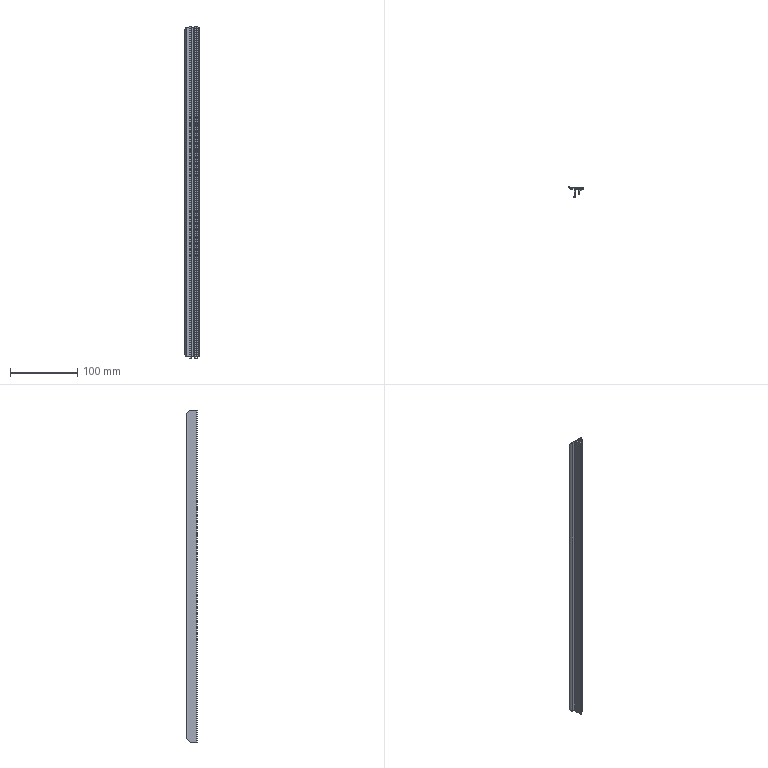Part | NX | features BREP 1 | 1 solid | 43 faces | box 21.266 x 16.173 x 494.9 mm | volume 33584 mm3 | plane 28 | cylinder 15 | commonest cylinder face diameters 0.585 x7 0.4 x2 1.951 x2 1.561 x1 8.16 x1 10.664 x1
STEP:
#1=CARTESIAN_POINT('',(0.,2.699,242.251));
#2=VERTEX_POINT('',#1);
#3=CARTESIAN_POINT('',(2.095,-0.55,245.5));
#4=VERTEX_POINT('',#3);
#5=CARTESIAN_POINT('',(0.,2.699,242.251));
#6=CARTESIAN_POINT('',(0.2706,1.376,243.574));
#7=CARTESIAN_POINT('',(1.002,0.242,244.708));
#8=CARTESIAN_POINT('',(2.095,-0.55,245.5));
#9=(BOUNDED_CURVE()B_SPLINE_CURVE(3,(#5,#6,#7,#8),.UNSPECIFIED.,.F.,.F.)B_SPLINE_CURVE_WITH_KNOTS((4,4),(1.773,2.515),.UNSPECIFIED.)CURVE()GEOMETRIC_REPRESENTATION_ITEM()RATIONAL_B_SPLINE_CURVE((1.,0.9547,0.9547,1.))REPRESENTATION_ITEM(''));
#10=EDGE_CURVE('',#2,#4,#9,.T.);
#11=ORIENTED_EDGE('',*,*,#10,.F.);
#12=CARTESIAN_POINT('',(0.,2.699,-242.251));
#13=VERTEX_POINT('',#12);
#14=CARTESIAN_POINT('',(0.,2.699,247.45));
#15=DIRECTION('',(0.,0.,-1.));
#16=VECTOR('',#15,1000.);
#17=LINE('',#14,#16);
#18=EDGE_CURVE('',#2,#13,#17,.T.);
#19=ORIENTED_EDGE('',*,*,#18,.T.);
#20=CARTESIAN_POINT('',(2.095,-0.55,-245.5));
#21=VERTEX_POINT('',#20);
#22=CARTESIAN_POINT('',(2.095,-0.55,-245.5));
#23=CARTESIAN_POINT('',(1.002,0.242,-244.708));
#24=CARTESIAN_POINT('',(0.2706,1.376,-243.574));
#25=CARTESIAN_POINT('',(0.,2.699,-242.251));
#26=(BOUNDED_CURVE()B_SPLINE_CURVE(3,(#22,#23,#24,#25),.UNSPECIFIED.,.F.,.F.)B_SPLINE_CURVE_WITH_KNOTS((4,4),(0.6271,1.369),.UNSPECIFIED.)CURVE()GEOMETRIC_REPRESENTATION_ITEM()RATIONAL_B_SPLINE_CURVE((1.,0.9547,0.9547,1.))REPRESENTATION_ITEM(''));
#27=EDGE_CURVE('',#21,#13,#26,.T.);
#28=ORIENTED_EDGE('',*,*,#27,.F.);
#29=CARTESIAN_POINT('',(2.095,-0.55,247.45));
#30=DIRECTION('',(0.,0.,-1.));
#31=VECTOR('',#30,1000.);
#32=LINE('',#29,#31);
#33=EDGE_CURVE('',#4,#21,#32,.T.);
#34=ORIENTED_EDGE('',*,*,#33,.F.);
#35=EDGE_LOOP('',(#11,#19,#28,#34));
#36=FACE_BOUND('',#35,.T.);
#37=CARTESIAN_POINT('',(5.224,3.768,247.45));
#38=DIRECTION('',(0.,0.,-1.));
#39=DIRECTION('',(-1.,0.,0.));
#40=AXIS2_PLACEMENT_3D('',#37,#38,#39);
#41=CYLINDRICAL_SURFACE('',#40,5.332);
#42=ADVANCED_FACE('',(#36),#41,.T.);
#43=CARTESIAN_POINT('',(7.9,-0.55,245.5));
#44=VERTEX_POINT('',#43);
#45=CARTESIAN_POINT('',(2.095,-0.55,245.5));
#46=DIRECTION('',(1.,0.,0.));
#47=VECTOR('',#46,1000.);
#48=LINE('',#45,#47);
#49=EDGE_CURVE('',#4,#44,#48,.T.);
#50=ORIENTED_EDGE('',*,*,#49,.F.);
#51=ORIENTED_EDGE('',*,*,#33,.T.);
#52=CARTESIAN_POINT('',(7.9,-0.55,-245.5));
#53=VERTEX_POINT('',#52);
#54=CARTESIAN_POINT('',(2.095,-0.55,-245.5));
#55=DIRECTION('',(-1.,0.,0.));
#56=VECTOR('',#55,1000.);
#57=LINE('',#54,#56);
#58=EDGE_CURVE('',#53,#21,#57,.T.);
#59=ORIENTED_EDGE('',*,*,#58,.F.);
#60=CARTESIAN_POINT('',(7.9,-0.55,247.45));
#61=DIRECTION('',(0.,0.,-1.));
#62=VECTOR('',#61,1000.);
#63=LINE('',#60,#62);
#64=EDGE_CURVE('',#44,#53,#63,.T.);
#65=ORIENTED_EDGE('',*,*,#64,.F.);
#66=EDGE_LOOP('',(#50,#51,#59,#65));
#67=FACE_BOUND('',#66,.T.);
#68=CARTESIAN_POINT('',(2.095,-0.55,247.45));
#69=DIRECTION('',(0.,1.,0.));
#70=DIRECTION('',(1.,0.,0.));
#71=AXIS2_PLACEMENT_3D('',#68,#69,#70);
#72=PLANE('',#71);
#73=ADVANCED_FACE('',(#67),#72,.F.);
#74=CARTESIAN_POINT('',(7.9,-2.5,247.45));
#75=VERTEX_POINT('',#74);
#76=CARTESIAN_POINT('',(7.9,-1.525,246.475));
#77=DIRECTION('',(0.,-0.7071,0.7071));
#78=VECTOR('',#77,1000.);
#79=LINE('',#76,#78);
#80=EDGE_CURVE('',#44,#75,#79,.T.);
#81=ORIENTED_EDGE('',*,*,#80,.F.);
#82=ORIENTED_EDGE('',*,*,#64,.T.);
#83=CARTESIAN_POINT('',(7.9,-2.5,-247.45));
#84=VERTEX_POINT('',#83);
#85=CARTESIAN_POINT('',(7.9,245.925,0.975));
#86=DIRECTION('',(0.,0.7071,0.7071));
#87=VECTOR('',#86,1000.);
#88=LINE('',#85,#87);
#89=EDGE_CURVE('',#84,#53,#88,.T.);
#90=ORIENTED_EDGE('',*,*,#89,.F.);
#91=CARTESIAN_POINT('',(7.9,-11.847,-247.45));
#92=VERTEX_POINT('',#91);
#93=CARTESIAN_POINT('',(7.9,-0.55,-247.45));
#94=DIRECTION('',(0.,-1.,0.));
#95=VECTOR('',#94,1000.);
#96=LINE('',#93,#95);
#97=EDGE_CURVE('',#84,#92,#96,.T.);
#98=ORIENTED_EDGE('',*,*,#97,.T.);
#99=CARTESIAN_POINT('',(7.9,-11.847,247.45));
#100=VERTEX_POINT('',#99);
#101=CARTESIAN_POINT('',(7.9,-11.847,247.45));
#102=DIRECTION('',(0.,0.,-1.));
#103=VECTOR('',#102,1000.);
#104=LINE('',#101,#103);
#105=EDGE_CURVE('',#100,#92,#104,.T.);
#106=ORIENTED_EDGE('',*,*,#105,.F.);
#107=CARTESIAN_POINT('',(7.9,-0.55,247.45));
#108=DIRECTION('',(0.,-1.,0.));
#109=VECTOR('',#108,1000.);
#110=LINE('',#107,#109);
#111=EDGE_CURVE('',#75,#100,#110,.T.);
#112=ORIENTED_EDGE('',*,*,#111,.F.);
#113=EDGE_LOOP('',(#81,#82,#90,#98,#106,#112));
#114=FACE_BOUND('',#113,.T.);
#115=CARTESIAN_POINT('',(7.9,-0.55,247.45));
#116=DIRECTION('',(1.,0.,0.));
#117=DIRECTION('',(0.,1.,0.));
#118=AXIS2_PLACEMENT_3D('',#115,#116,#117);
#119=PLANE('',#118);
#120=ADVANCED_FACE('',(#114),#119,.F.);
#121=CARTESIAN_POINT('',(9.363,-2.5,247.45));
#122=VERTEX_POINT('',#121);
#123=CARTESIAN_POINT('',(9.363,-1.526,246.476));
#124=VERTEX_POINT('',#123);
#125=CARTESIAN_POINT('',(9.363,-7.399,252.349));
#126=DIRECTION('',(0.,0.7071,-0.7071));
#127=VECTOR('',#126,1000.);
#128=LINE('',#125,#127);
#129=EDGE_CURVE('',#122,#124,#128,.T.);
#130=ORIENTED_EDGE('',*,*,#129,.F.);
#131=CARTESIAN_POINT('',(9.363,-12.298,247.45));
#132=VERTEX_POINT('',#131);
#133=CARTESIAN_POINT('',(9.363,-12.298,247.45));
#134=DIRECTION('',(0.,1.,0.));
#135=VECTOR('',#134,1000.);
#136=LINE('',#133,#135);
#137=EDGE_CURVE('',#132,#122,#136,.T.);
#138=ORIENTED_EDGE('',*,*,#137,.F.);
#139=CARTESIAN_POINT('',(9.363,-12.298,-247.45));
#140=VERTEX_POINT('',#139);
#141=CARTESIAN_POINT('',(9.363,-12.298,247.45));
#142=DIRECTION('',(0.,0.,-1.));
#143=VECTOR('',#142,1000.);
#144=LINE('',#141,#143);
#145=EDGE_CURVE('',#132,#140,#144,.T.);
#146=ORIENTED_EDGE('',*,*,#145,.T.);
#147=CARTESIAN_POINT('',(9.363,-2.5,-247.45));
#148=VERTEX_POINT('',#147);
#149=CARTESIAN_POINT('',(9.363,-12.298,-247.45));
#150=DIRECTION('',(0.,1.,0.));
#151=VECTOR('',#150,1000.);
#152=LINE('',#149,#151);
#153=EDGE_CURVE('',#140,#148,#152,.T.);
#154=ORIENTED_EDGE('',*,*,#153,.T.);
#155=CARTESIAN_POINT('',(9.363,-1.526,-246.476));
#156=VERTEX_POINT('',#155);
#157=CARTESIAN_POINT('',(9.363,240.051,-4.899));
#158=DIRECTION('',(0.,-0.7071,-0.7071));
#159=VECTOR('',#158,1000.);
#160=LINE('',#157,#159);
#161=EDGE_CURVE('',#156,#148,#160,.T.);
#162=ORIENTED_EDGE('',*,*,#161,.F.);
#163=CARTESIAN_POINT('',(9.363,-1.526,247.45));
#164=DIRECTION('',(0.,0.,-1.));
#165=VECTOR('',#164,1000.);
#166=LINE('',#163,#165);
#167=EDGE_CURVE('',#124,#156,#166,.T.);
#168=ORIENTED_EDGE('',*,*,#167,.F.);
#169=EDGE_LOOP('',(#130,#138,#146,#154,#162,#168));
#170=FACE_BOUND('',#169,.T.);
#171=CARTESIAN_POINT('',(9.363,-12.298,247.45));
#172=DIRECTION('',(-1.,0.,0.));
#173=DIRECTION('',(0.,0.,1.));
#174=AXIS2_PLACEMENT_3D('',#171,#172,#173);
#175=PLANE('',#174);
#176=ADVANCED_FACE('',(#170),#175,.F.);
#177=CARTESIAN_POINT('',(10.339,-0.55,245.5));
#178=VERTEX_POINT('',#177);
#179=CARTESIAN_POINT('',(9.363,-1.526,246.476));
#180=CARTESIAN_POINT('',(9.363,-0.9541,245.904));
#181=CARTESIAN_POINT('',(9.768,-0.55,245.5));
#182=CARTESIAN_POINT('',(10.339,-0.55,245.5));
#183=(BOUNDED_CURVE()B_SPLINE_CURVE(3,(#179,#180,#181,#182),.UNSPECIFIED.,.F.,.F.)B_SPLINE_CURVE_WITH_KNOTS((4,4),(4.712,6.283),.UNSPECIFIED.)CURVE()GEOMETRIC_REPRESENTATION_ITEM()RATIONAL_B_SPLINE_CURVE((1.,0.8047,0.8047,1.))REPRESENTATION_ITEM(''));
#184=EDGE_CURVE('',#124,#178,#183,.T.);
#185=ORIENTED_EDGE('',*,*,#184,.F.);
#186=ORIENTED_EDGE('',*,*,#167,.T.);
#187=CARTESIAN_POINT('',(10.339,-0.55,-245.5));
#188=VERTEX_POINT('',#187);
#189=CARTESIAN_POINT('',(10.339,-0.55,-245.5));
#190=CARTESIAN_POINT('',(9.768,-0.55,-245.5));
#191=CARTESIAN_POINT('',(9.363,-0.9541,-245.904));
#192=CARTESIAN_POINT('',(9.363,-1.526,-246.476));
#193=(BOUNDED_CURVE()B_SPLINE_CURVE(3,(#189,#190,#191,#192),.UNSPECIFIED.,.F.,.F.)B_SPLINE_CURVE_WITH_KNOTS((4,4),(3.142,4.712),.UNSPECIFIED.)CURVE()GEOMETRIC_REPRESENTATION_ITEM()RATIONAL_B_SPLINE_CURVE((1.,0.8047,0.8047,1.))REPRESENTATION_ITEM(''));
#194=EDGE_CURVE('',#188,#156,#193,.T.);
#195=ORIENTED_EDGE('',*,*,#194,.F.);
#196=CARTESIAN_POINT('',(10.339,-0.55,247.45));
#197=DIRECTION('',(0.,0.,-1.));
#198=VECTOR('',#197,1000.);
#199=LINE('',#196,#198);
#200=EDGE_CURVE('',#178,#188,#199,.T.);
#201=ORIENTED_EDGE('',*,*,#200,.F.);
#202=EDGE_LOOP('',(#185,#186,#195,#201));
#203=FACE_BOUND('',#202,.T.);
#204=CARTESIAN_POINT('',(10.339,-1.526,247.45));
#205=DIRECTION('',(0.,0.,-1.));
#206=DIRECTION('',(-1.,0.,0.));
#207=AXIS2_PLACEMENT_3D('',#204,#205,#206);
#208=CYLINDRICAL_SURFACE('',#207,0.9756);
#209=ADVANCED_FACE('',(#203),#208,.F.);
#210=CARTESIAN_POINT('',(13.461,-0.55,245.5));
#211=VERTEX_POINT('',#210);
#212=CARTESIAN_POINT('',(10.339,-0.55,245.5));
#213=DIRECTION('',(1.,0.,0.));
#214=VECTOR('',#213,1000.);
#215=LINE('',#212,#214);
#216=EDGE_CURVE('',#178,#211,#215,.T.);
#217=ORIENTED_EDGE('',*,*,#216,.F.);
#218=ORIENTED_EDGE('',*,*,#200,.T.);
#219=CARTESIAN_POINT('',(13.461,-0.55,-245.5));
#220=VERTEX_POINT('',#219);
#221=CARTESIAN_POINT('',(10.339,-0.55,-245.5));
#222=DIRECTION('',(-1.,0.,0.));
#223=VECTOR('',#222,1000.);
#224=LINE('',#221,#223);
#225=EDGE_CURVE('',#220,#188,#224,.T.);
#226=ORIENTED_EDGE('',*,*,#225,.F.);
#227=CARTESIAN_POINT('',(13.461,-0.55,247.45));
#228=DIRECTION('',(0.,0.,-1.));
#229=VECTOR('',#228,1000.);
#230=LINE('',#227,#229);
#231=EDGE_CURVE('',#211,#220,#230,.T.);
#232=ORIENTED_EDGE('',*,*,#231,.F.);
#233=EDGE_LOOP('',(#217,#218,#226,#232));
#234=FACE_BOUND('',#233,.T.);
#235=CARTESIAN_POINT('',(10.339,-0.55,247.45));
#236=DIRECTION('',(0.,1.,0.));
#237=DIRECTION('',(1.,0.,0.));
#238=AXIS2_PLACEMENT_3D('',#235,#236,#237);
#239=PLANE('',#238);
#240=ADVANCED_FACE('',(#234),#239,.F.);
#241=CARTESIAN_POINT('',(14.437,-1.526,246.476));
#242=VERTEX_POINT('',#241);
#243=CARTESIAN_POINT('',(13.461,-0.55,245.5));
#244=CARTESIAN_POINT('',(14.032,-0.55,245.5));
#245=CARTESIAN_POINT('',(14.437,-0.9541,245.904));
#246=CARTESIAN_POINT('',(14.437,-1.526,246.476));
#247=(BOUNDED_CURVE()B_SPLINE_CURVE(3,(#243,#244,#245,#246),.UNSPECIFIED.,.F.,.F.)B_SPLINE_CURVE_WITH_KNOTS((4,4),(0.,1.571),.UNSPECIFIED.)CURVE()GEOMETRIC_REPRESENTATION_ITEM()RATIONAL_B_SPLINE_CURVE((1.,0.8047,0.8047,1.))REPRESENTATION_ITEM(''));
#248=EDGE_CURVE('',#211,#242,#247,.T.);
#249=ORIENTED_EDGE('',*,*,#248,.F.);
#250=ORIENTED_EDGE('',*,*,#231,.T.);
#251=CARTESIAN_POINT('',(14.437,-1.526,-246.476));
#252=VERTEX_POINT('',#251);
#253=CARTESIAN_POINT('',(14.437,-1.526,-246.476));
#254=CARTESIAN_POINT('',(14.437,-0.9541,-245.904));
#255=CARTESIAN_POINT('',(14.032,-0.55,-245.5));
#256=CARTESIAN_POINT('',(13.461,-0.55,-245.5));
#257=(BOUNDED_CURVE()B_SPLINE_CURVE(3,(#253,#254,#255,#256),.UNSPECIFIED.,.F.,.F.)B_SPLINE_CURVE_WITH_KNOTS((4,4),(1.571,3.142),.UNSPECIFIED.)CURVE()GEOMETRIC_REPRESENTATION_ITEM()RATIONAL_B_SPLINE_CURVE((1.,0.8047,0.8047,1.))REPRESENTATION_ITEM(''));
#258=EDGE_CURVE('',#252,#220,#257,.T.);
#259=ORIENTED_EDGE('',*,*,#258,.F.);
#260=CARTESIAN_POINT('',(14.437,-1.526,247.45));
#261=DIRECTION('',(0.,0.,-1.));
#262=VECTOR('',#261,1000.);
#263=LINE('',#260,#262);
#264=EDGE_CURVE('',#242,#252,#263,.T.);
#265=ORIENTED_EDGE('',*,*,#264,.F.);
#266=EDGE_LOOP('',(#249,#250,#259,#265));
#267=FACE_BOUND('',#266,.T.);
#268=CARTESIAN_POINT('',(13.461,-1.526,247.45));
#269=DIRECTION('',(0.,0.,-1.));
#270=DIRECTION('',(-1.,0.,0.));
#271=AXIS2_PLACEMENT_3D('',#268,#269,#270);
#272=CYLINDRICAL_SURFACE('',#271,0.9756);
#273=ADVANCED_FACE('',(#267),#272,.F.);
#274=CARTESIAN_POINT('',(14.437,-2.5,247.45));
#275=VERTEX_POINT('',#274);
#276=CARTESIAN_POINT('',(14.437,-2.013,246.963));
#277=DIRECTION('',(0.,-0.7071,0.7071));
#278=VECTOR('',#277,1000.);
#279=LINE('',#276,#278);
#280=EDGE_CURVE('',#242,#275,#279,.T.);
#281=ORIENTED_EDGE('',*,*,#280,.F.);
#282=ORIENTED_EDGE('',*,*,#264,.T.);
#283=CARTESIAN_POINT('',(14.437,-2.5,-247.45));
#284=VERTEX_POINT('',#283);
#285=CARTESIAN_POINT('',(14.437,245.437,0.4872));
#286=DIRECTION('',(0.,0.7071,0.7071));
#287=VECTOR('',#286,1000.);
#288=LINE('',#285,#287);
#289=EDGE_CURVE('',#284,#252,#288,.T.);
#290=ORIENTED_EDGE('',*,*,#289,.F.);
#291=CARTESIAN_POINT('',(14.437,-8.128,-247.45));
#292=VERTEX_POINT('',#291);
#293=CARTESIAN_POINT('',(14.437,-1.526,-247.45));
#294=DIRECTION('',(0.,-1.,0.));
#295=VECTOR('',#294,1000.);
#296=LINE('',#293,#295);
#297=EDGE_CURVE('',#284,#292,#296,.T.);
#298=ORIENTED_EDGE('',*,*,#297,.T.);
#299=CARTESIAN_POINT('',(14.437,-8.128,247.45));
#300=VERTEX_POINT('',#299);
#301=CARTESIAN_POINT('',(14.437,-8.128,247.45));
#302=DIRECTION('',(0.,0.,-1.));
#303=VECTOR('',#302,1000.);
#304=LINE('',#301,#303);
#305=EDGE_CURVE('',#300,#292,#304,.T.);
#306=ORIENTED_EDGE('',*,*,#305,.F.);
#307=CARTESIAN_POINT('',(14.437,-1.526,247.45));
#308=DIRECTION('',(0.,-1.,0.));
#309=VECTOR('',#308,1000.);
#310=LINE('',#307,#309);
#311=EDGE_CURVE('',#275,#300,#310,.T.);
#312=ORIENTED_EDGE('',*,*,#311,.F.);
#313=EDGE_LOOP('',(#281,#282,#290,#298,#306,#312));
#314=FACE_BOUND('',#313,.T.);
#315=CARTESIAN_POINT('',(14.437,-1.526,247.45));
#316=DIRECTION('',(1.,0.,0.));
#317=DIRECTION('',(0.,1.,0.));
#318=AXIS2_PLACEMENT_3D('',#315,#316,#317);
#319=PLANE('',#318);
#320=ADVANCED_FACE('',(#314),#319,.F.);
#321=CARTESIAN_POINT('',(15.9,-2.5,247.45));
#322=VERTEX_POINT('',#321);
#323=CARTESIAN_POINT('',(15.9,-0.55,245.5));
#324=VERTEX_POINT('',#323);
#325=CARTESIAN_POINT('',(15.9,-4.93,249.88));
#326=DIRECTION('',(0.,0.7071,-0.7071));
#327=VECTOR('',#326,1000.);
#328=LINE('',#325,#327);
#329=EDGE_CURVE('',#322,#324,#328,.T.);
#330=ORIENTED_EDGE('',*,*,#329,.F.);
#331=CARTESIAN_POINT('',(15.9,-7.36,247.45));
#332=VERTEX_POINT('',#331);
#333=CARTESIAN_POINT('',(15.9,-7.36,247.45));
#334=DIRECTION('',(0.,1.,0.));
#335=VECTOR('',#334,1000.);
#336=LINE('',#333,#335);
#337=EDGE_CURVE('',#332,#322,#336,.T.);
#338=ORIENTED_EDGE('',*,*,#337,.F.);
#339=CARTESIAN_POINT('',(15.9,-7.36,-247.45));
#340=VERTEX_POINT('',#339);
#341=CARTESIAN_POINT('',(15.9,-7.36,247.45));
#342=DIRECTION('',(0.,0.,-1.));
#343=VECTOR('',#342,1000.);
#344=LINE('',#341,#343);
#345=EDGE_CURVE('',#332,#340,#344,.T.);
#346=ORIENTED_EDGE('',*,*,#345,.T.);
#347=CARTESIAN_POINT('',(15.9,-2.5,-247.45));
#348=VERTEX_POINT('',#347);
#349=CARTESIAN_POINT('',(15.9,-7.36,-247.45));
#350=DIRECTION('',(0.,1.,0.));
#351=VECTOR('',#350,1000.);
#352=LINE('',#349,#351);
#353=EDGE_CURVE('',#340,#348,#352,.T.);
#354=ORIENTED_EDGE('',*,*,#353,.T.);
#355=CARTESIAN_POINT('',(15.9,-0.55,-245.5));
#356=VERTEX_POINT('',#355);
#357=CARTESIAN_POINT('',(15.9,242.52,-2.43));
#358=DIRECTION('',(0.,-0.7071,-0.7071));
#359=VECTOR('',#358,1000.);
#360=LINE('',#357,#359);
#361=EDGE_CURVE('',#356,#348,#360,.T.);
#362=ORIENTED_EDGE('',*,*,#361,.F.);
#363=CARTESIAN_POINT('',(15.9,-0.55,247.45));
#364=DIRECTION('',(0.,0.,-1.));
#365=VECTOR('',#364,1000.);
#366=LINE('',#363,#365);
#367=EDGE_CURVE('',#324,#356,#366,.T.);
#368=ORIENTED_EDGE('',*,*,#367,.F.);
#369=EDGE_LOOP('',(#330,#338,#346,#354,#362,#368));
#370=FACE_BOUND('',#369,.T.);
#371=CARTESIAN_POINT('',(15.9,-7.36,247.45));
#372=DIRECTION('',(-1.,0.,0.));
#373=DIRECTION('',(0.,0.,1.));
#374=AXIS2_PLACEMENT_3D('',#371,#372,#373);
#375=PLANE('',#374);
#376=ADVANCED_FACE('',(#370),#375,.F.);
#377=CARTESIAN_POINT('',(17.363,-0.55,245.5));
#378=VERTEX_POINT('',#377);
#379=CARTESIAN_POINT('',(15.9,-0.55,245.5));
#380=DIRECTION('',(1.,0.,0.));
#381=VECTOR('',#380,1000.);
#382=LINE('',#379,#381);
#383=EDGE_CURVE('',#324,#378,#382,.T.);
#384=ORIENTED_EDGE('',*,*,#383,.F.);
#385=ORIENTED_EDGE('',*,*,#367,.T.);
#386=CARTESIAN_POINT('',(17.363,-0.55,-245.5));
#387=VERTEX_POINT('',#386);
#388=CARTESIAN_POINT('',(15.9,-0.55,-245.5));
#389=DIRECTION('',(-1.,0.,0.));
#390=VECTOR('',#389,1000.);
#391=LINE('',#388,#390);
#392=EDGE_CURVE('',#387,#356,#391,.T.);
#393=ORIENTED_EDGE('',*,*,#392,.F.);
#394=CARTESIAN_POINT('',(17.363,-0.55,247.45));
#395=DIRECTION('',(0.,0.,-1.));
#396=VECTOR('',#395,1000.);
#397=LINE('',#394,#396);
#398=EDGE_CURVE('',#378,#387,#397,.T.);
#399=ORIENTED_EDGE('',*,*,#398,.F.);
#400=EDGE_LOOP('',(#384,#385,#393,#399));
#401=FACE_BOUND('',#400,.T.);
#402=CARTESIAN_POINT('',(15.9,-0.55,247.45));
#403=DIRECTION('',(0.,1.,0.));
#404=DIRECTION('',(1.,0.,0.));
#405=AXIS2_PLACEMENT_3D('',#402,#403,#404);
#406=PLANE('',#405);
#407=ADVANCED_FACE('',(#401),#406,.F.);
#408=CARTESIAN_POINT('',(17.363,-2.5,247.45));
#409=VERTEX_POINT('',#408);
#410=CARTESIAN_POINT('',(17.363,-1.525,246.475));
#411=DIRECTION('',(0.,-0.7071,0.7071));
#412=VECTOR('',#411,1000.);
#413=LINE('',#410,#412);
#414=EDGE_CURVE('',#378,#409,#413,.T.);
#415=ORIENTED_EDGE('',*,*,#414,.F.);
#416=ORIENTED_EDGE('',*,*,#398,.T.);
#417=CARTESIAN_POINT('',(17.363,-2.5,-247.45));
#418=VERTEX_POINT('',#417);
#419=CARTESIAN_POINT('',(17.363,245.925,0.975));
#420=DIRECTION('',(0.,0.7071,0.7071));
#421=VECTOR('',#420,1000.);
#422=LINE('',#419,#421);
#423=EDGE_CURVE('',#418,#387,#422,.T.);
#424=ORIENTED_EDGE('',*,*,#423,.F.);
#425=CARTESIAN_POINT('',(17.363,-2.501,-247.45));
#426=VERTEX_POINT('',#425);
#427=CARTESIAN_POINT('',(17.363,-0.55,-247.45));
#428=DIRECTION('',(0.,-1.,0.));
#429=VECTOR('',#428,1000.);
#430=LINE('',#427,#429);
#431=EDGE_CURVE('',#418,#426,#430,.T.);
#432=ORIENTED_EDGE('',*,*,#431,.T.);
#433=CARTESIAN_POINT('',(17.363,-2.501,247.45));
#434=VERTEX_POINT('',#433);
#435=CARTESIAN_POINT('',(17.363,-2.501,247.45));
#436=DIRECTION('',(0.,0.,-1.));
#437=VECTOR('',#436,1000.);
#438=LINE('',#435,#437);
#439=EDGE_CURVE('',#434,#426,#438,.T.);
#440=ORIENTED_EDGE('',*,*,#439,.F.);
#441=CARTESIAN_POINT('',(17.363,-0.55,247.45));
#442=DIRECTION('',(0.,-1.,0.));
#443=VECTOR('',#442,1000.);
#444=LINE('',#441,#443);
#445=EDGE_CURVE('',#409,#434,#444,.T.);
#446=ORIENTED_EDGE('',*,*,#445,.F.);
#447=EDGE_LOOP('',(#415,#416,#424,#432,#440,#446));
#448=FACE_BOUND('',#447,.T.);
#449=CARTESIAN_POINT('',(17.363,-0.55,247.45));
#450=DIRECTION('',(1.,0.,0.));
#451=DIRECTION('',(0.,1.,0.));
#452=AXIS2_PLACEMENT_3D('',#449,#450,#451);
#453=PLANE('',#452);
#454=ADVANCED_FACE('',(#448),#453,.F.);
#455=CARTESIAN_POINT('',(19.049,-2.5,247.45));
#456=VERTEX_POINT('',#455);
#457=CARTESIAN_POINT('',(19.315,-2.209,247.159));
#458=VERTEX_POINT('',#457);
#459=CARTESIAN_POINT('',(19.049,-2.5,247.45));
#460=CARTESIAN_POINT('',(19.207,-2.485,247.435));
#461=CARTESIAN_POINT('',(19.315,-2.368,247.318));
#462=CARTESIAN_POINT('',(19.315,-2.209,247.159));
#463=(BOUNDED_CURVE()B_SPLINE_CURVE(3,(#459,#460,#461,#462),.UNSPECIFIED.,.F.,.F.)B_SPLINE_CURVE_WITH_KNOTS((4,4),(3.233,4.712),.UNSPECIFIED.)CURVE()GEOMETRIC_REPRESENTATION_ITEM()RATIONAL_B_SPLINE_CURVE((1.,0.8258,0.8258,1.))REPRESENTATION_ITEM(''));
#464=EDGE_CURVE('',#456,#458,#463,.T.);
#465=ORIENTED_EDGE('',*,*,#464,.F.);
#466=CARTESIAN_POINT('',(19.022,-2.501,247.45));
#467=VERTEX_POINT('',#466);
#468=CARTESIAN_POINT('',(19.022,-2.209,247.45));
#469=DIRECTION('',(0.,0.,1.));
#470=DIRECTION('',(1.,0.,0.));
#471=AXIS2_PLACEMENT_3D('',#468,#469,#470);
#472=CIRCLE('',#471,0.2927);
#473=EDGE_CURVE('',#467,#456,#472,.T.);
#474=ORIENTED_EDGE('',*,*,#473,.F.);
#475=CARTESIAN_POINT('',(19.022,-2.501,-247.45));
#476=VERTEX_POINT('',#475);
#477=CARTESIAN_POINT('',(19.022,-2.501,247.45));
#478=DIRECTION('',(0.,0.,-1.));
#479=VECTOR('',#478,1000.);
#480=LINE('',#477,#479);
#481=EDGE_CURVE('',#467,#476,#480,.T.);
#482=ORIENTED_EDGE('',*,*,#481,.T.);
#483=CARTESIAN_POINT('',(19.049,-2.5,-247.45));
#484=VERTEX_POINT('',#483);
#485=CARTESIAN_POINT('',(19.022,-2.209,-247.45));
#486=DIRECTION('',(0.,0.,1.));
#487=DIRECTION('',(1.,0.,0.));
#488=AXIS2_PLACEMENT_3D('',#485,#486,#487);
#489=CIRCLE('',#488,0.2927);
#490=EDGE_CURVE('',#476,#484,#489,.T.);
#491=ORIENTED_EDGE('',*,*,#490,.T.);
#492=CARTESIAN_POINT('',(19.315,-2.209,-247.159));
#493=VERTEX_POINT('',#492);
#494=CARTESIAN_POINT('',(19.315,-2.209,-247.159));
#495=CARTESIAN_POINT('',(19.315,-2.368,-247.318));
#496=CARTESIAN_POINT('',(19.207,-2.485,-247.435));
#497=CARTESIAN_POINT('',(19.049,-2.5,-247.45));
#498=(BOUNDED_CURVE()B_SPLINE_CURVE(3,(#494,#495,#496,#497),.UNSPECIFIED.,.F.,.F.)B_SPLINE_CURVE_WITH_KNOTS((4,4),(4.712,6.192),.UNSPECIFIED.)CURVE()GEOMETRIC_REPRESENTATION_ITEM()RATIONAL_B_SPLINE_CURVE((1.,0.8258,0.8258,1.))REPRESENTATION_ITEM(''));
#499=EDGE_CURVE('',#493,#484,#498,.T.);
#500=ORIENTED_EDGE('',*,*,#499,.F.);
#501=CARTESIAN_POINT('',(19.315,-2.209,247.45));
#502=DIRECTION('',(0.,0.,-1.));
#503=VECTOR('',#502,1000.);
#504=LINE('',#501,#503);
#505=EDGE_CURVE('',#458,#493,#504,.T.);
#506=ORIENTED_EDGE('',*,*,#505,.F.);
#507=EDGE_LOOP('',(#465,#474,#482,#491,#500,#506));
#508=FACE_BOUND('',#507,.T.);
#509=CARTESIAN_POINT('',(19.022,-2.209,247.45));
#510=DIRECTION('',(0.,0.,-1.));
#511=DIRECTION('',(-1.,0.,0.));
#512=AXIS2_PLACEMENT_3D('',#509,#510,#511);
#513=CYLINDRICAL_SURFACE('',#512,0.2927);
#514=ADVANCED_FACE('',(#508),#513,.T.);
#515=CARTESIAN_POINT('',(19.315,-0.8427,245.793));
#516=VERTEX_POINT('',#515);
#517=CARTESIAN_POINT('',(19.315,-2.354,247.304));
#518=DIRECTION('',(0.,0.7071,-0.7071));
#519=VECTOR('',#518,1000.);
#520=LINE('',#517,#519);
#521=EDGE_CURVE('',#458,#516,#520,.T.);
#522=ORIENTED_EDGE('',*,*,#521,.F.);
#523=ORIENTED_EDGE('',*,*,#505,.T.);
#524=CARTESIAN_POINT('',(19.315,-0.8427,-245.793));
#525=VERTEX_POINT('',#524);
#526=CARTESIAN_POINT('',(19.315,245.096,0.1457));
#527=DIRECTION('',(0.,-0.7071,-0.7071));
#528=VECTOR('',#527,1000.);
#529=LINE('',#526,#528);
#530=EDGE_CURVE('',#525,#493,#529,.T.);
#531=ORIENTED_EDGE('',*,*,#530,.F.);
#532=CARTESIAN_POINT('',(19.315,-0.8427,247.45));
#533=DIRECTION('',(0.,0.,-1.));
#534=VECTOR('',#533,1000.);
#535=LINE('',#532,#534);
#536=EDGE_CURVE('',#516,#525,#535,.T.);
#537=ORIENTED_EDGE('',*,*,#536,.F.);
#538=EDGE_LOOP('',(#522,#523,#531,#537));
#539=FACE_BOUND('',#538,.T.);
#540=CARTESIAN_POINT('',(19.315,-2.209,247.45));
#541=DIRECTION('',(-1.,0.,0.));
#542=DIRECTION('',(0.,0.,1.));
#543=AXIS2_PLACEMENT_3D('',#540,#541,#542);
#544=PLANE('',#543);
#545=ADVANCED_FACE('',(#539),#544,.F.);
#546=CARTESIAN_POINT('',(19.607,-0.55,245.5));
#547=VERTEX_POINT('',#546);
#548=CARTESIAN_POINT('',(19.315,-0.8427,245.793));
#549=CARTESIAN_POINT('',(19.315,-0.6712,245.621));
#550=CARTESIAN_POINT('',(19.436,-0.55,245.5));
#551=CARTESIAN_POINT('',(19.607,-0.55,245.5));
#552=(BOUNDED_CURVE()B_SPLINE_CURVE(3,(#548,#549,#550,#551),.UNSPECIFIED.,.F.,.F.)B_SPLINE_CURVE_WITH_KNOTS((4,4),(4.712,6.283),.UNSPECIFIED.)CURVE()GEOMETRIC_REPRESENTATION_ITEM()RATIONAL_B_SPLINE_CURVE((1.,0.8047,0.8047,1.))REPRESENTATION_ITEM(''));
#553=EDGE_CURVE('',#516,#547,#552,.T.);
#554=ORIENTED_EDGE('',*,*,#553,.F.);
#555=ORIENTED_EDGE('',*,*,#536,.T.);
#556=CARTESIAN_POINT('',(19.607,-0.55,-245.5));
#557=VERTEX_POINT('',#556);
#558=CARTESIAN_POINT('',(19.607,-0.55,-245.5));
#559=CARTESIAN_POINT('',(19.436,-0.55,-245.5));
#560=CARTESIAN_POINT('',(19.315,-0.6712,-245.621));
#561=CARTESIAN_POINT('',(19.315,-0.8427,-245.793));
#562=(BOUNDED_CURVE()B_SPLINE_CURVE(3,(#558,#559,#560,#561),.UNSPECIFIED.,.F.,.F.)B_SPLINE_CURVE_WITH_KNOTS((4,4),(3.142,4.712),.UNSPECIFIED.)CURVE()GEOMETRIC_REPRESENTATION_ITEM()RATIONAL_B_SPLINE_CURVE((1.,0.8047,0.8047,1.))REPRESENTATION_ITEM(''));
#563=EDGE_CURVE('',#557,#525,#562,.T.);
#564=ORIENTED_EDGE('',*,*,#563,.F.);
#565=CARTESIAN_POINT('',(19.607,-0.55,247.45));
#566=DIRECTION('',(0.,0.,-1.));
#567=VECTOR('',#566,1000.);
#568=LINE('',#565,#567);
#569=EDGE_CURVE('',#547,#557,#568,.T.);
#570=ORIENTED_EDGE('',*,*,#569,.F.);
#571=EDGE_LOOP('',(#554,#555,#564,#570));
#572=FACE_BOUND('',#571,.T.);
#573=CARTESIAN_POINT('',(19.607,-0.8427,247.45));
#574=DIRECTION('',(0.,0.,-1.));
#575=DIRECTION('',(-1.,0.,0.));
#576=AXIS2_PLACEMENT_3D('',#573,#574,#575);
#577=CYLINDRICAL_SURFACE('',#576,0.2927);
#578=ADVANCED_FACE('',(#572),#577,.F.);
#579=CARTESIAN_POINT('',(20.973,-0.55,245.5));
#580=VERTEX_POINT('',#579);
#581=CARTESIAN_POINT('',(19.607,-0.55,245.5));
#582=DIRECTION('',(1.,0.,0.));
#583=VECTOR('',#582,1000.);
#584=LINE('',#581,#583);
#585=EDGE_CURVE('',#547,#580,#584,.T.);
#586=ORIENTED_EDGE('',*,*,#585,.F.);
#587=ORIENTED_EDGE('',*,*,#569,.T.);
#588=CARTESIAN_POINT('',(20.973,-0.55,-245.5));
#589=VERTEX_POINT('',#588);
#590=CARTESIAN_POINT('',(19.607,-0.55,-245.5));
#591=DIRECTION('',(-1.,0.,0.));
#592=VECTOR('',#591,1000.);
#593=LINE('',#590,#592);
#594=EDGE_CURVE('',#589,#557,#593,.T.);
#595=ORIENTED_EDGE('',*,*,#594,.F.);
#596=CARTESIAN_POINT('',(20.973,-0.55,247.45));
#597=DIRECTION('',(0.,0.,-1.));
#598=VECTOR('',#597,1000.);
#599=LINE('',#596,#598);
#600=EDGE_CURVE('',#580,#589,#599,.T.);
#601=ORIENTED_EDGE('',*,*,#600,.F.);
#602=EDGE_LOOP('',(#586,#587,#595,#601));
#603=FACE_BOUND('',#602,.T.);
#604=CARTESIAN_POINT('',(19.607,-0.55,247.45));
#605=DIRECTION('',(0.,1.,0.));
#606=DIRECTION('',(1.,0.,0.));
#607=AXIS2_PLACEMENT_3D('',#604,#605,#606);
#608=PLANE('',#607);
#609=ADVANCED_FACE('',(#603),#608,.F.);
#610=CARTESIAN_POINT('',(21.266,-0.2573,245.207));
#611=VERTEX_POINT('',#610);
#612=CARTESIAN_POINT('',(20.973,-0.55,245.5));
#613=CARTESIAN_POINT('',(21.145,-0.55,245.5));
#614=CARTESIAN_POINT('',(21.266,-0.4288,245.379));
#615=CARTESIAN_POINT('',(21.266,-0.2573,245.207));
#616=(BOUNDED_CURVE()B_SPLINE_CURVE(3,(#612,#613,#614,#615),.UNSPECIFIED.,.F.,.F.)B_SPLINE_CURVE_WITH_KNOTS((4,4),(3.142,4.712),.UNSPECIFIED.)CURVE()GEOMETRIC_REPRESENTATION_ITEM()RATIONAL_B_SPLINE_CURVE((1.,0.8047,0.8047,1.))REPRESENTATION_ITEM(''));
#617=EDGE_CURVE('',#580,#611,#616,.T.);
#618=ORIENTED_EDGE('',*,*,#617,.F.);
#619=ORIENTED_EDGE('',*,*,#600,.T.);
#620=CARTESIAN_POINT('',(21.266,-0.2573,-245.207));
#621=VERTEX_POINT('',#620);
#622=CARTESIAN_POINT('',(21.266,-0.2573,-245.207));
#623=CARTESIAN_POINT('',(21.266,-0.4288,-245.379));
#624=CARTESIAN_POINT('',(21.145,-0.55,-245.5));
#625=CARTESIAN_POINT('',(20.973,-0.55,-245.5));
#626=(BOUNDED_CURVE()B_SPLINE_CURVE(3,(#622,#623,#624,#625),.UNSPECIFIED.,.F.,.F.)B_SPLINE_CURVE_WITH_KNOTS((4,4),(4.712,6.283),.UNSPECIFIED.)CURVE()GEOMETRIC_REPRESENTATION_ITEM()RATIONAL_B_SPLINE_CURVE((1.,0.8047,0.8047,1.))REPRESENTATION_ITEM(''));
#627=EDGE_CURVE('',#621,#589,#626,.T.);
#628=ORIENTED_EDGE('',*,*,#627,.F.);
#629=CARTESIAN_POINT('',(21.266,-0.2573,247.45));
#630=DIRECTION('',(0.,0.,-1.));
#631=VECTOR('',#630,1000.);
#632=LINE('',#629,#631);
#633=EDGE_CURVE('',#611,#621,#632,.T.);
#634=ORIENTED_EDGE('',*,*,#633,.F.);
#635=EDGE_LOOP('',(#618,#619,#628,#634));
#636=FACE_BOUND('',#635,.T.);
#637=CARTESIAN_POINT('',(20.973,-0.2573,247.45));
#638=DIRECTION('',(0.,0.,-1.));
#639=DIRECTION('',(-1.,0.,0.));
#640=AXIS2_PLACEMENT_3D('',#637,#638,#639);
#641=CYLINDRICAL_SURFACE('',#640,0.2927);
#642=ADVANCED_FACE('',(#636),#641,.T.);
#643=CARTESIAN_POINT('',(21.266,0.8034,244.147));
#644=VERTEX_POINT('',#643);
#645=CARTESIAN_POINT('',(21.266,-2.5,247.45));
#646=DIRECTION('',(0.,0.7071,-0.7071));
#647=VECTOR('',#646,1000.);
#648=LINE('',#645,#647);
#649=EDGE_CURVE('',#611,#644,#648,.T.);
#650=ORIENTED_EDGE('',*,*,#649,.F.);
#651=ORIENTED_EDGE('',*,*,#633,.T.);
#652=CARTESIAN_POINT('',(21.266,0.8034,-244.147));
#653=VERTEX_POINT('',#652);
#654=CARTESIAN_POINT('',(21.266,-2.5,-247.45));
#655=DIRECTION('',(0.,-0.7071,-0.7071));
#656=VECTOR('',#655,1000.);
#657=LINE('',#654,#656);
#658=EDGE_CURVE('',#653,#621,#657,.T.);
#659=ORIENTED_EDGE('',*,*,#658,.F.);
#660=CARTESIAN_POINT('',(21.266,0.8034,247.45));
#661=DIRECTION('',(0.,0.,-1.));
#662=VECTOR('',#661,1000.);
#663=LINE('',#660,#662);
#664=EDGE_CURVE('',#644,#653,#663,.T.);
#665=ORIENTED_EDGE('',*,*,#664,.F.);
#666=EDGE_LOOP('',(#650,#651,#659,#665));
#667=FACE_BOUND('',#666,.T.);
#668=CARTESIAN_POINT('',(21.266,-0.2573,247.45));
#669=DIRECTION('',(-1.,0.,0.));
#670=DIRECTION('',(0.,0.,1.));
#671=AXIS2_PLACEMENT_3D('',#668,#669,#670);
#672=PLANE('',#671);
#673=ADVANCED_FACE('',(#667),#672,.F.);
#674=CARTESIAN_POINT('',(21.066,1.003,243.947));
#675=VERTEX_POINT('',#674);
#676=CARTESIAN_POINT('',(21.266,0.8034,244.147));
#677=CARTESIAN_POINT('',(21.266,0.9206,244.029));
#678=CARTESIAN_POINT('',(21.183,1.003,243.947));
#679=CARTESIAN_POINT('',(21.066,1.003,243.947));
#680=(BOUNDED_CURVE()B_SPLINE_CURVE(3,(#676,#677,#678,#679),.UNSPECIFIED.,.F.,.F.)B_SPLINE_CURVE_WITH_KNOTS((4,4),(4.712,6.283),.UNSPECIFIED.)CURVE()GEOMETRIC_REPRESENTATION_ITEM()RATIONAL_B_SPLINE_CURVE((1.,0.8047,0.8047,1.))REPRESENTATION_ITEM(''));
#681=EDGE_CURVE('',#644,#675,#680,.T.);
#682=ORIENTED_EDGE('',*,*,#681,.F.);
#683=ORIENTED_EDGE('',*,*,#664,.T.);
#684=CARTESIAN_POINT('',(21.066,1.003,-243.947));
#685=VERTEX_POINT('',#684);
#686=CARTESIAN_POINT('',(21.066,1.003,-243.947));
#687=CARTESIAN_POINT('',(21.183,1.003,-243.947));
#688=CARTESIAN_POINT('',(21.266,0.9206,-244.029));
#689=CARTESIAN_POINT('',(21.266,0.8034,-244.147));
#690=(BOUNDED_CURVE()B_SPLINE_CURVE(3,(#686,#687,#688,#689),.UNSPECIFIED.,.F.,.F.)B_SPLINE_CURVE_WITH_KNOTS((4,4),(3.142,4.712),.UNSPECIFIED.)CURVE()GEOMETRIC_REPRESENTATION_ITEM()RATIONAL_B_SPLINE_CURVE((1.,0.8047,0.8047,1.))REPRESENTATION_ITEM(''));
#691=EDGE_CURVE('',#685,#653,#690,.T.);
#692=ORIENTED_EDGE('',*,*,#691,.F.);
#693=CARTESIAN_POINT('',(21.066,1.003,247.45));
#694=DIRECTION('',(0.,0.,-1.));
#695=VECTOR('',#694,1000.);
#696=LINE('',#693,#695);
#697=EDGE_CURVE('',#675,#685,#696,.T.);
#698=ORIENTED_EDGE('',*,*,#697,.F.);
#699=EDGE_LOOP('',(#682,#683,#692,#698));
#700=FACE_BOUND('',#699,.T.);
#701=CARTESIAN_POINT('',(21.066,0.8034,247.45));
#702=DIRECTION('',(0.,0.,-1.));
#703=DIRECTION('',(-1.,0.,0.));
#704=AXIS2_PLACEMENT_3D('',#701,#702,#703);
#705=CYLINDRICAL_SURFACE('',#704,0.2);
#706=ADVANCED_FACE('',(#700),#705,.T.);
#707=CARTESIAN_POINT('',(3.014,1.003,243.947));
#708=VERTEX_POINT('',#707);
#709=CARTESIAN_POINT('',(21.066,1.003,243.947));
#710=DIRECTION('',(-1.,0.,0.));
#711=VECTOR('',#710,1000.);
#712=LINE('',#709,#711);
#713=EDGE_CURVE('',#675,#708,#712,.T.);
#714=ORIENTED_EDGE('',*,*,#713,.F.);
#715=ORIENTED_EDGE('',*,*,#697,.T.);
#716=CARTESIAN_POINT('',(3.014,1.003,-243.947));
#717=VERTEX_POINT('',#716);
#718=CARTESIAN_POINT('',(21.066,1.003,-243.947));
#719=DIRECTION('',(1.,0.,0.));
#720=VECTOR('',#719,1000.);
#721=LINE('',#718,#720);
#722=EDGE_CURVE('',#717,#685,#721,.T.);
#723=ORIENTED_EDGE('',*,*,#722,.F.);
#724=CARTESIAN_POINT('',(3.014,1.003,247.45));
#725=DIRECTION('',(0.,0.,-1.));
#726=VECTOR('',#725,1000.);
#727=LINE('',#724,#726);
#728=EDGE_CURVE('',#708,#717,#727,.T.);
#729=ORIENTED_EDGE('',*,*,#728,.F.);
#730=EDGE_LOOP('',(#714,#715,#723,#729));
#731=FACE_BOUND('',#730,.T.);
#732=CARTESIAN_POINT('',(21.066,1.003,247.45));
#733=DIRECTION('',(0.,-1.,0.));
#734=DIRECTION('',(0.,0.,-1.));
#735=AXIS2_PLACEMENT_3D('',#732,#733,#734);
#736=PLANE('',#735);
#737=ADVANCED_FACE('',(#731),#736,.F.);
#738=CARTESIAN_POINT('',(0.3705,2.864,242.086));
#739=VERTEX_POINT('',#738);
#740=CARTESIAN_POINT('',(3.014,1.003,243.947));
#741=CARTESIAN_POINT('',(1.898,1.237,243.713));
#742=CARTESIAN_POINT('',(0.9663,1.892,243.058));
#743=CARTESIAN_POINT('',(0.3705,2.864,242.086));
#744=(BOUNDED_CURVE()B_SPLINE_CURVE(3,(#740,#741,#742,#743),.UNSPECIFIED.,.F.,.F.)B_SPLINE_CURVE_WITH_KNOTS((4,4),(3.348,4.162),.UNSPECIFIED.)CURVE()GEOMETRIC_REPRESENTATION_ITEM()RATIONAL_B_SPLINE_CURVE((1.,0.9455,0.9455,1.))REPRESENTATION_ITEM(''));
#745=EDGE_CURVE('',#708,#739,#744,.T.);
#746=ORIENTED_EDGE('',*,*,#745,.F.);
#747=ORIENTED_EDGE('',*,*,#728,.T.);
#748=CARTESIAN_POINT('',(0.3705,2.864,-242.086));
#749=VERTEX_POINT('',#748);
#750=CARTESIAN_POINT('',(0.3705,2.864,-242.086));
#751=CARTESIAN_POINT('',(0.9663,1.892,-243.058));
#752=CARTESIAN_POINT('',(1.898,1.237,-243.713));
#753=CARTESIAN_POINT('',(3.014,1.003,-243.947));
#754=(BOUNDED_CURVE()B_SPLINE_CURVE(3,(#750,#751,#752,#753),.UNSPECIFIED.,.F.,.F.)B_SPLINE_CURVE_WITH_KNOTS((4,4),(5.263,6.077),.UNSPECIFIED.)CURVE()GEOMETRIC_REPRESENTATION_ITEM()RATIONAL_B_SPLINE_CURVE((1.,0.9455,0.9455,1.))REPRESENTATION_ITEM(''));
#755=EDGE_CURVE('',#749,#717,#754,.T.);
#756=ORIENTED_EDGE('',*,*,#755,.F.);
#757=CARTESIAN_POINT('',(0.3705,2.864,247.45));
#758=DIRECTION('',(0.,0.,-1.));
#759=VECTOR('',#758,1000.);
#760=LINE('',#757,#759);
#761=EDGE_CURVE('',#739,#749,#760,.T.);
#762=ORIENTED_EDGE('',*,*,#761,.F.);
#763=EDGE_LOOP('',(#746,#747,#756,#762));
#764=FACE_BOUND('',#763,.T.);
#765=CARTESIAN_POINT('',(3.848,4.997,247.45));
#766=DIRECTION('',(0.,0.,-1.));
#767=DIRECTION('',(-1.,0.,0.));
#768=AXIS2_PLACEMENT_3D('',#765,#766,#767);
#769=CYLINDRICAL_SURFACE('',#768,4.08);
#770=ADVANCED_FACE('',(#764),#769,.F.);
#771=CARTESIAN_POINT('',(0.,2.759,242.191));
#772=VERTEX_POINT('',#771);
#773=CARTESIAN_POINT('',(0.,2.759,-242.191));
#774=VERTEX_POINT('',#773);
#775=CARTESIAN_POINT('',(0.,2.759,247.45));
#776=DIRECTION('',(0.,0.,-1.));
#777=VECTOR('',#776,1000.);
#778=LINE('',#775,#777);
#779=EDGE_CURVE('',#772,#774,#778,.T.);
#780=ORIENTED_EDGE('',*,*,#779,.F.);
#781=CARTESIAN_POINT('',(0.3705,2.864,242.086));
#782=CARTESIAN_POINT('',(0.2401,3.077,241.873));
#783=CARTESIAN_POINT('',(0.,3.009,241.941));
#784=CARTESIAN_POINT('',(0.,2.759,242.191));
#785=(BOUNDED_CURVE()B_SPLINE_CURVE(3,(#781,#782,#783,#784),.UNSPECIFIED.,.F.,.F.)B_SPLINE_CURVE_WITH_KNOTS((4,4),(5.263,7.854),.UNSPECIFIED.)CURVE()GEOMETRIC_REPRESENTATION_ITEM()RATIONAL_B_SPLINE_CURVE((1.,0.5144,0.5144,1.))REPRESENTATION_ITEM(''));
#786=EDGE_CURVE('',#739,#772,#785,.T.);
#787=ORIENTED_EDGE('',*,*,#786,.F.);
#788=ORIENTED_EDGE('',*,*,#761,.T.);
#789=CARTESIAN_POINT('',(0.,2.759,-242.191));
#790=CARTESIAN_POINT('',(0.,3.009,-241.941));
#791=CARTESIAN_POINT('',(0.2401,3.077,-241.873));
#792=CARTESIAN_POINT('',(0.3705,2.864,-242.086));
#793=(BOUNDED_CURVE()B_SPLINE_CURVE(3,(#789,#790,#791,#792),.UNSPECIFIED.,.F.,.F.)B_SPLINE_CURVE_WITH_KNOTS((4,4),(1.571,4.162),.UNSPECIFIED.)CURVE()GEOMETRIC_REPRESENTATION_ITEM()RATIONAL_B_SPLINE_CURVE((1.,0.5144,0.5144,1.))REPRESENTATION_ITEM(''));
#794=EDGE_CURVE('',#774,#749,#793,.T.);
#795=ORIENTED_EDGE('',*,*,#794,.F.);
#796=EDGE_LOOP('',(#780,#787,#788,#795));
#797=FACE_BOUND('',#796,.T.);
#798=CARTESIAN_POINT('',(0.2,2.759,247.45));
#799=DIRECTION('',(0.,0.,-1.));
#800=DIRECTION('',(-1.,0.,0.));
#801=AXIS2_PLACEMENT_3D('',#798,#799,#800);
#802=CYLINDRICAL_SURFACE('',#801,0.2);
#803=ADVANCED_FACE('',(#797),#802,.T.);
#804=CARTESIAN_POINT('',(0.,-2.5,247.45));
#805=DIRECTION('',(0.,0.7071,-0.7071));
#806=VECTOR('',#805,1000.);
#807=LINE('',#804,#806);
#808=EDGE_CURVE('',#2,#772,#807,.T.);
#809=ORIENTED_EDGE('',*,*,#808,.T.);
#810=ORIENTED_EDGE('',*,*,#779,.T.);
#811=CARTESIAN_POINT('',(0.,-2.5,-247.45));
#812=DIRECTION('',(0.,-0.7071,-0.7071));
#813=VECTOR('',#812,1000.);
#814=LINE('',#811,#813);
#815=EDGE_CURVE('',#774,#13,#814,.T.);
#816=ORIENTED_EDGE('',*,*,#815,.T.);
#817=ORIENTED_EDGE('',*,*,#18,.F.);
#818=EDGE_LOOP('',(#809,#810,#816,#817));
#819=FACE_BOUND('',#818,.T.);
#820=CARTESIAN_POINT('',(0.,2.759,247.45));
#821=DIRECTION('',(1.,0.,0.));
#822=DIRECTION('',(0.,1.,0.));
#823=AXIS2_PLACEMENT_3D('',#820,#821,#822);
#824=PLANE('',#823);
#825=ADVANCED_FACE('',(#819),#824,.F.);
#826=ORIENTED_EDGE('',*,*,#473,.T.);
#827=CARTESIAN_POINT('',(5.224,-2.5,247.45));
#828=DIRECTION('',(-1.,0.,0.));
#829=VECTOR('',#828,1000.);
#830=LINE('',#827,#829);
#831=EDGE_CURVE('',#456,#409,#830,.T.);
#832=ORIENTED_EDGE('',*,*,#831,.T.);
#833=ORIENTED_EDGE('',*,*,#445,.T.);
#834=CARTESIAN_POINT('',(17.363,-2.501,247.45));
#835=DIRECTION('',(1.,0.,0.));
#836=VECTOR('',#835,1000.);
#837=LINE('',#834,#836);
#838=EDGE_CURVE('',#434,#467,#837,.T.);
#839=ORIENTED_EDGE('',*,*,#838,.T.);
#840=EDGE_LOOP('',(#826,#832,#833,#839));
#841=FACE_BOUND('',#840,.T.);
#842=CARTESIAN_POINT('',(5.224,3.768,247.45));
#843=DIRECTION('',(0.,0.,1.));
#844=DIRECTION('',(1.,0.,0.));
#845=AXIS2_PLACEMENT_3D('',#842,#843,#844);
#846=PLANE('',#845);
#847=ADVANCED_FACE('',(#841),#846,.T.);
#848=ORIENTED_EDGE('',*,*,#337,.T.);
#849=CARTESIAN_POINT('',(5.224,-2.5,247.45));
#850=DIRECTION('',(-1.,0.,0.));
#851=VECTOR('',#850,1000.);
#852=LINE('',#849,#851);
#853=EDGE_CURVE('',#322,#275,#852,.T.);
#854=ORIENTED_EDGE('',*,*,#853,.T.);
#855=ORIENTED_EDGE('',*,*,#311,.T.);
#856=CARTESIAN_POINT('',(15.719,-8.726,247.45));
#857=VERTEX_POINT('',#856);
#858=CARTESIAN_POINT('',(15.217,-8.128,247.45));
#859=DIRECTION('',(0.,0.,1.));
#860=DIRECTION('',(1.,0.,0.));
#861=AXIS2_PLACEMENT_3D('',#858,#859,#860);
#862=CIRCLE('',#861,0.7805);
#863=EDGE_CURVE('',#300,#857,#862,.T.);
#864=ORIENTED_EDGE('',*,*,#863,.T.);
#865=CARTESIAN_POINT('',(16.381,-8.171,247.45));
#866=VERTEX_POINT('',#865);
#867=CARTESIAN_POINT('',(15.719,-8.726,247.45));
#868=DIRECTION('',(0.766,0.6428,0.));
#869=VECTOR('',#868,1000.);
#870=LINE('',#867,#869);
#871=EDGE_CURVE('',#857,#866,#870,.T.);
#872=ORIENTED_EDGE('',*,*,#871,.T.);
#873=CARTESIAN_POINT('',(16.485,-7.946,247.45));
#874=VERTEX_POINT('',#873);
#875=CARTESIAN_POINT('',(16.193,-7.946,247.45));
#876=DIRECTION('',(0.,0.,1.));
#877=DIRECTION('',(1.,0.,0.));
#878=AXIS2_PLACEMENT_3D('',#875,#876,#877);
#879=CIRCLE('',#878,0.2927);
#880=EDGE_CURVE('',#866,#874,#879,.T.);
#881=ORIENTED_EDGE('',*,*,#880,.T.);
#882=CARTESIAN_POINT('',(16.485,-7.652,247.45));
#883=VERTEX_POINT('',#882);
#884=CARTESIAN_POINT('',(16.485,-7.946,247.45));
#885=DIRECTION('',(0.,1.,0.));
#886=VECTOR('',#885,1000.);
#887=LINE('',#884,#886);
#888=EDGE_CURVE('',#874,#883,#887,.T.);
#889=ORIENTED_EDGE('',*,*,#888,.T.);
#890=CARTESIAN_POINT('',(16.193,-7.36,247.45));
#891=VERTEX_POINT('',#890);
#892=CARTESIAN_POINT('',(16.193,-7.652,247.45));
#893=DIRECTION('',(0.,0.,1.));
#894=DIRECTION('',(1.,0.,0.));
#895=AXIS2_PLACEMENT_3D('',#892,#893,#894);
#896=CIRCLE('',#895,0.2927);
#897=EDGE_CURVE('',#883,#891,#896,.T.);
#898=ORIENTED_EDGE('',*,*,#897,.T.);
#899=CARTESIAN_POINT('',(16.193,-7.36,247.45));
#900=DIRECTION('',(-1.,0.,0.));
#901=VECTOR('',#900,1000.);
#902=LINE('',#899,#901);
#903=EDGE_CURVE('',#891,#332,#902,.T.);
#904=ORIENTED_EDGE('',*,*,#903,.T.);
#905=EDGE_LOOP('',(#848,#854,#855,#864,#872,#881,#889,#898,#904));
#906=FACE_BOUND('',#905,.T.);
#907=CARTESIAN_POINT('',(5.224,3.768,247.45));
#908=DIRECTION('',(0.,0.,1.));
#909=DIRECTION('',(1.,0.,0.));
#910=AXIS2_PLACEMENT_3D('',#907,#908,#909);
#911=PLANE('',#910);
#912=ADVANCED_FACE('',(#906),#911,.T.);
#913=ORIENTED_EDGE('',*,*,#137,.T.);
#914=CARTESIAN_POINT('',(5.224,-2.5,247.45));
#915=DIRECTION('',(-1.,0.,0.));
#916=VECTOR('',#915,1000.);
#917=LINE('',#914,#916);
#918=EDGE_CURVE('',#122,#75,#917,.T.);
#919=ORIENTED_EDGE('',*,*,#918,.T.);
#920=ORIENTED_EDGE('',*,*,#111,.T.);
#921=CARTESIAN_POINT('',(7.607,-11.847,247.45));
#922=VERTEX_POINT('',#921);
#923=CARTESIAN_POINT('',(7.9,-11.847,247.45));
#924=DIRECTION('',(-1.,0.,0.));
#925=VECTOR('',#924,1000.);
#926=LINE('',#923,#925);
#927=EDGE_CURVE('',#100,#922,#926,.T.);
#928=ORIENTED_EDGE('',*,*,#927,.T.);
#929=CARTESIAN_POINT('',(7.315,-12.14,247.45));
#930=VERTEX_POINT('',#929);
#931=CARTESIAN_POINT('',(7.607,-12.14,247.45));
#932=DIRECTION('',(0.,0.,1.));
#933=DIRECTION('',(1.,0.,0.));
#934=AXIS2_PLACEMENT_3D('',#931,#932,#933);
#935=CIRCLE('',#934,0.2927);
#936=EDGE_CURVE('',#922,#930,#935,.T.);
#937=ORIENTED_EDGE('',*,*,#936,.T.);
#938=CARTESIAN_POINT('',(7.315,-12.434,247.45));
#939=VERTEX_POINT('',#938);
#940=CARTESIAN_POINT('',(7.315,-12.14,247.45));
#941=DIRECTION('',(0.,-1.,0.));
#942=VECTOR('',#941,1000.);
#943=LINE('',#940,#942);
#944=EDGE_CURVE('',#930,#939,#943,.T.);
#945=ORIENTED_EDGE('',*,*,#944,.T.);
#946=CARTESIAN_POINT('',(7.419,-12.658,247.45));
#947=VERTEX_POINT('',#946);
#948=CARTESIAN_POINT('',(7.607,-12.434,247.45));
#949=DIRECTION('',(0.,0.,1.));
#950=DIRECTION('',(1.,0.,0.));
#951=AXIS2_PLACEMENT_3D('',#948,#949,#950);
#952=CIRCLE('',#951,0.2927);
#953=EDGE_CURVE('',#939,#947,#952,.T.);
#954=ORIENTED_EDGE('',*,*,#953,.T.);
#955=CARTESIAN_POINT('',(8.081,-13.214,247.45));
#956=VERTEX_POINT('',#955);
#957=CARTESIAN_POINT('',(7.419,-12.658,247.45));
#958=DIRECTION('',(0.766,-0.6428,0.));
#959=VECTOR('',#958,1000.);
#960=LINE('',#957,#959);
#961=EDGE_CURVE('',#947,#956,#960,.T.);
#962=ORIENTED_EDGE('',*,*,#961,.T.);
#963=CARTESIAN_POINT('',(0.,-0.55,247.45));
#964=DIRECTION('',(0.,0.,1.));
#965=DIRECTION('',(1.,0.,0.));
#966=AXIS2_PLACEMENT_3D('',#963,#964,#965);
#967=CIRCLE('',#966,15.023);
#968=EDGE_CURVE('',#956,#132,#967,.T.);
#969=ORIENTED_EDGE('',*,*,#968,.T.);
#970=EDGE_LOOP('',(#913,#919,#920,#928,#937,#945,#954,#962,#969));
#971=FACE_BOUND('',#970,.T.);
#972=CARTESIAN_POINT('',(5.224,3.768,247.45));
#973=DIRECTION('',(0.,0.,1.));
#974=DIRECTION('',(1.,0.,0.));
#975=AXIS2_PLACEMENT_3D('',#972,#973,#974);
#976=PLANE('',#975);
#977=ADVANCED_FACE('',(#971),#976,.T.);
#978=CARTESIAN_POINT('',(5.224,-2.5,-247.45));
#979=DIRECTION('',(-1.,0.,0.));
#980=VECTOR('',#979,1000.);
#981=LINE('',#978,#980);
#982=EDGE_CURVE('',#484,#418,#981,.T.);
#983=ORIENTED_EDGE('',*,*,#982,.F.);
#984=ORIENTED_EDGE('',*,*,#490,.F.);
#985=CARTESIAN_POINT('',(17.363,-2.501,-247.45));
#986=DIRECTION('',(1.,0.,0.));
#987=VECTOR('',#986,1000.);
#988=LINE('',#985,#987);
#989=EDGE_CURVE('',#426,#476,#988,.T.);
#990=ORIENTED_EDGE('',*,*,#989,.F.);
#991=ORIENTED_EDGE('',*,*,#431,.F.);
#992=EDGE_LOOP('',(#983,#984,#990,#991));
#993=FACE_BOUND('',#992,.T.);
#994=CARTESIAN_POINT('',(5.224,3.768,-247.45));
#995=DIRECTION('',(0.,0.,1.));
#996=DIRECTION('',(1.,0.,0.));
#997=AXIS2_PLACEMENT_3D('',#994,#995,#996);
#998=PLANE('',#997);
#999=ADVANCED_FACE('',(#993),#998,.F.);
#1000=CARTESIAN_POINT('',(5.224,-2.5,-247.45));
#1001=DIRECTION('',(-1.,0.,0.));
#1002=VECTOR('',#1001,1000.);
#1003=LINE('',#1000,#1002);
#1004=EDGE_CURVE('',#348,#284,#1003,.T.);
#1005=ORIENTED_EDGE('',*,*,#1004,.F.);
#1006=ORIENTED_EDGE('',*,*,#353,.F.);
#1007=CARTESIAN_POINT('',(16.193,-7.36,-247.45));
#1008=VERTEX_POINT('',#1007);
#1009=CARTESIAN_POINT('',(16.193,-7.36,-247.45));
#1010=DIRECTION('',(-1.,0.,0.));
#1011=VECTOR('',#1010,1000.);
#1012=LINE('',#1009,#1011);
#1013=EDGE_CURVE('',#1008,#340,#1012,.T.);
#1014=ORIENTED_EDGE('',*,*,#1013,.F.);
#1015=CARTESIAN_POINT('',(16.485,-7.652,-247.45));
#1016=VERTEX_POINT('',#1015);
#1017=CARTESIAN_POINT('',(16.193,-7.652,-247.45));
#1018=DIRECTION('',(0.,0.,1.));
#1019=DIRECTION('',(1.,0.,0.));
#1020=AXIS2_PLACEMENT_3D('',#1017,#1018,#1019);
#1021=CIRCLE('',#1020,0.2927);
#1022=EDGE_CURVE('',#1016,#1008,#1021,.T.);
#1023=ORIENTED_EDGE('',*,*,#1022,.F.);
#1024=CARTESIAN_POINT('',(16.485,-7.946,-247.45));
#1025=VERTEX_POINT('',#1024);
#1026=CARTESIAN_POINT('',(16.485,-7.946,-247.45));
#1027=DIRECTION('',(0.,1.,0.));
#1028=VECTOR('',#1027,1000.);
#1029=LINE('',#1026,#1028);
#1030=EDGE_CURVE('',#1025,#1016,#1029,.T.);
#1031=ORIENTED_EDGE('',*,*,#1030,.F.);
#1032=CARTESIAN_POINT('',(16.381,-8.171,-247.45));
#1033=VERTEX_POINT('',#1032);
#1034=CARTESIAN_POINT('',(16.193,-7.946,-247.45));
#1035=DIRECTION('',(0.,0.,1.));
#1036=DIRECTION('',(1.,0.,0.));
#1037=AXIS2_PLACEMENT_3D('',#1034,#1035,#1036);
#1038=CIRCLE('',#1037,0.2927);
#1039=EDGE_CURVE('',#1033,#1025,#1038,.T.);
#1040=ORIENTED_EDGE('',*,*,#1039,.F.);
#1041=CARTESIAN_POINT('',(15.719,-8.726,-247.45));
#1042=VERTEX_POINT('',#1041);
#1043=CARTESIAN_POINT('',(15.719,-8.726,-247.45));
#1044=DIRECTION('',(0.766,0.6428,0.));
#1045=VECTOR('',#1044,1000.);
#1046=LINE('',#1043,#1045);
#1047=EDGE_CURVE('',#1042,#1033,#1046,.T.);
#1048=ORIENTED_EDGE('',*,*,#1047,.F.);
#1049=CARTESIAN_POINT('',(15.217,-8.128,-247.45));
#1050=DIRECTION('',(0.,0.,1.));
#1051=DIRECTION('',(1.,0.,0.));
#1052=AXIS2_PLACEMENT_3D('',#1049,#1050,#1051);
#1053=CIRCLE('',#1052,0.7805);
#1054=EDGE_CURVE('',#292,#1042,#1053,.T.);
#1055=ORIENTED_EDGE('',*,*,#1054,.F.);
#1056=ORIENTED_EDGE('',*,*,#297,.F.);
#1057=EDGE_LOOP('',(#1005,#1006,#1014,#1023,#1031,#1040,#1048,#1055,#1056));
#1058=FACE_BOUND('',#1057,.T.);
#1059=CARTESIAN_POINT('',(5.224,3.768,-247.45));
#1060=DIRECTION('',(0.,0.,1.));
#1061=DIRECTION('',(1.,0.,0.));
#1062=AXIS2_PLACEMENT_3D('',#1059,#1060,#1061);
#1063=PLANE('',#1062);
#1064=ADVANCED_FACE('',(#1058),#1063,.F.);
#1065=CARTESIAN_POINT('',(5.224,-2.5,-247.45));
#1066=DIRECTION('',(-1.,0.,0.));
#1067=VECTOR('',#1066,1000.);
#1068=LINE('',#1065,#1067);
#1069=EDGE_CURVE('',#148,#84,#1068,.T.);
#1070=ORIENTED_EDGE('',*,*,#1069,.F.);
#1071=ORIENTED_EDGE('',*,*,#153,.F.);
#1072=CARTESIAN_POINT('',(8.081,-13.214,-247.45));
#1073=VERTEX_POINT('',#1072);
#1074=CARTESIAN_POINT('',(0.,-0.55,-247.45));
#1075=DIRECTION('',(0.,0.,1.));
#1076=DIRECTION('',(1.,0.,0.));
#1077=AXIS2_PLACEMENT_3D('',#1074,#1075,#1076);
#1078=CIRCLE('',#1077,15.023);
#1079=EDGE_CURVE('',#1073,#140,#1078,.T.);
#1080=ORIENTED_EDGE('',*,*,#1079,.F.);
#1081=CARTESIAN_POINT('',(7.419,-12.658,-247.45));
#1082=VERTEX_POINT('',#1081);
#1083=CARTESIAN_POINT('',(7.419,-12.658,-247.45));
#1084=DIRECTION('',(0.766,-0.6428,0.));
#1085=VECTOR('',#1084,1000.);
#1086=LINE('',#1083,#1085);
#1087=EDGE_CURVE('',#1082,#1073,#1086,.T.);
#1088=ORIENTED_EDGE('',*,*,#1087,.F.);
#1089=CARTESIAN_POINT('',(7.315,-12.434,-247.45));
#1090=VERTEX_POINT('',#1089);
#1091=CARTESIAN_POINT('',(7.607,-12.434,-247.45));
#1092=DIRECTION('',(0.,0.,1.));
#1093=DIRECTION('',(1.,0.,0.));
#1094=AXIS2_PLACEMENT_3D('',#1091,#1092,#1093);
#1095=CIRCLE('',#1094,0.2927);
#1096=EDGE_CURVE('',#1090,#1082,#1095,.T.);
#1097=ORIENTED_EDGE('',*,*,#1096,.F.);
#1098=CARTESIAN_POINT('',(7.315,-12.14,-247.45));
#1099=VERTEX_POINT('',#1098);
#1100=CARTESIAN_POINT('',(7.315,-12.14,-247.45));
#1101=DIRECTION('',(0.,-1.,0.));
#1102=VECTOR('',#1101,1000.);
#1103=LINE('',#1100,#1102);
#1104=EDGE_CURVE('',#1099,#1090,#1103,.T.);
#1105=ORIENTED_EDGE('',*,*,#1104,.F.);
#1106=CARTESIAN_POINT('',(7.607,-11.847,-247.45));
#1107=VERTEX_POINT('',#1106);
#1108=CARTESIAN_POINT('',(7.607,-12.14,-247.45));
#1109=DIRECTION('',(0.,0.,1.));
#1110=DIRECTION('',(1.,0.,0.));
#1111=AXIS2_PLACEMENT_3D('',#1108,#1109,#1110);
#1112=CIRCLE('',#1111,0.2927);
#1113=EDGE_CURVE('',#1107,#1099,#1112,.T.);
#1114=ORIENTED_EDGE('',*,*,#1113,.F.);
#1115=CARTESIAN_POINT('',(7.9,-11.847,-247.45));
#1116=DIRECTION('',(-1.,0.,0.));
#1117=VECTOR('',#1116,1000.);
#1118=LINE('',#1115,#1117);
#1119=EDGE_CURVE('',#92,#1107,#1118,.T.);
#1120=ORIENTED_EDGE('',*,*,#1119,.F.);
#1121=ORIENTED_EDGE('',*,*,#97,.F.);
#1122=EDGE_LOOP('',(#1070,#1071,#1080,#1088,#1097,#1105,#1114,#1120,#1121));
#1123=FACE_BOUND('',#1122,.T.);
#1124=CARTESIAN_POINT('',(5.224,3.768,-247.45));
#1125=DIRECTION('',(0.,0.,1.));
#1126=DIRECTION('',(1.,0.,0.));
#1127=AXIS2_PLACEMENT_3D('',#1124,#1125,#1126);
#1128=PLANE('',#1127);
#1129=ADVANCED_FACE('',(#1123),#1128,.F.);
#1130=ORIENTED_EDGE('',*,*,#1119,.T.);
#1131=CARTESIAN_POINT('',(7.607,-11.847,247.45));
#1132=DIRECTION('',(0.,0.,-1.));
#1133=VECTOR('',#1132,1000.);
#1134=LINE('',#1131,#1133);
#1135=EDGE_CURVE('',#922,#1107,#1134,.T.);
#1136=ORIENTED_EDGE('',*,*,#1135,.F.);
#1137=ORIENTED_EDGE('',*,*,#927,.F.);
#1138=ORIENTED_EDGE('',*,*,#105,.T.);
#1139=EDGE_LOOP('',(#1130,#1136,#1137,#1138));
#1140=FACE_BOUND('',#1139,.T.);
#1141=CARTESIAN_POINT('',(7.9,-11.847,247.45));
#1142=DIRECTION('',(0.,-1.,0.));
#1143=DIRECTION('',(0.,0.,-1.));
#1144=AXIS2_PLACEMENT_3D('',#1141,#1142,#1143);
#1145=PLANE('',#1144);
#1146=ADVANCED_FACE('',(#1140),#1145,.F.);
#1147=ORIENTED_EDGE('',*,*,#1113,.T.);
#1148=CARTESIAN_POINT('',(7.315,-12.14,247.45));
#1149=DIRECTION('',(0.,0.,-1.));
#1150=VECTOR('',#1149,1000.);
#1151=LINE('',#1148,#1150);
#1152=EDGE_CURVE('',#930,#1099,#1151,.T.);
#1153=ORIENTED_EDGE('',*,*,#1152,.F.);
#1154=ORIENTED_EDGE('',*,*,#936,.F.);
#1155=ORIENTED_EDGE('',*,*,#1135,.T.);
#1156=EDGE_LOOP('',(#1147,#1153,#1154,#1155));
#1157=FACE_BOUND('',#1156,.T.);
#1158=CARTESIAN_POINT('',(7.607,-12.14,247.45));
#1159=DIRECTION('',(0.,0.,-1.));
#1160=DIRECTION('',(-1.,0.,0.));
#1161=AXIS2_PLACEMENT_3D('',#1158,#1159,#1160);
#1162=CYLINDRICAL_SURFACE('',#1161,0.2927);
#1163=ADVANCED_FACE('',(#1157),#1162,.T.);
#1164=ORIENTED_EDGE('',*,*,#1104,.T.);
#1165=CARTESIAN_POINT('',(7.315,-12.434,247.45));
#1166=DIRECTION('',(0.,0.,-1.));
#1167=VECTOR('',#1166,1000.);
#1168=LINE('',#1165,#1167);
#1169=EDGE_CURVE('',#939,#1090,#1168,.T.);
#1170=ORIENTED_EDGE('',*,*,#1169,.F.);
#1171=ORIENTED_EDGE('',*,*,#944,.F.);
#1172=ORIENTED_EDGE('',*,*,#1152,.T.);
#1173=EDGE_LOOP('',(#1164,#1170,#1171,#1172));
#1174=FACE_BOUND('',#1173,.T.);
#1175=CARTESIAN_POINT('',(7.315,-12.14,247.45));
#1176=DIRECTION('',(1.,0.,0.));
#1177=DIRECTION('',(0.,1.,0.));
#1178=AXIS2_PLACEMENT_3D('',#1175,#1176,#1177);
#1179=PLANE('',#1178);
#1180=ADVANCED_FACE('',(#1174),#1179,.F.);
#1181=ORIENTED_EDGE('',*,*,#1096,.T.);
#1182=CARTESIAN_POINT('',(7.419,-12.658,247.45));
#1183=DIRECTION('',(0.,0.,-1.));
#1184=VECTOR('',#1183,1000.);
#1185=LINE('',#1182,#1184);
#1186=EDGE_CURVE('',#947,#1082,#1185,.T.);
#1187=ORIENTED_EDGE('',*,*,#1186,.F.);
#1188=ORIENTED_EDGE('',*,*,#953,.F.);
#1189=ORIENTED_EDGE('',*,*,#1169,.T.);
#1190=EDGE_LOOP('',(#1181,#1187,#1188,#1189));
#1191=FACE_BOUND('',#1190,.T.);
#1192=CARTESIAN_POINT('',(7.607,-12.434,247.45));
#1193=DIRECTION('',(0.,0.,-1.));
#1194=DIRECTION('',(-1.,0.,0.));
#1195=AXIS2_PLACEMENT_3D('',#1192,#1193,#1194);
#1196=CYLINDRICAL_SURFACE('',#1195,0.2927);
#1197=ADVANCED_FACE('',(#1191),#1196,.T.);
#1198=ORIENTED_EDGE('',*,*,#1087,.T.);
#1199=CARTESIAN_POINT('',(8.081,-13.214,247.45));
#1200=DIRECTION('',(0.,0.,-1.));
#1201=VECTOR('',#1200,1000.);
#1202=LINE('',#1199,#1201);
#1203=EDGE_CURVE('',#956,#1073,#1202,.T.);
#1204=ORIENTED_EDGE('',*,*,#1203,.F.);
#1205=ORIENTED_EDGE('',*,*,#961,.F.);
#1206=ORIENTED_EDGE('',*,*,#1186,.T.);
#1207=EDGE_LOOP('',(#1198,#1204,#1205,#1206));
#1208=FACE_BOUND('',#1207,.T.);
#1209=CARTESIAN_POINT('',(7.419,-12.658,247.45));
#1210=DIRECTION('',(0.6428,0.766,0.));
#1211=DIRECTION('',(0.,0.,-1.));
#1212=AXIS2_PLACEMENT_3D('',#1209,#1210,#1211);
#1213=PLANE('',#1212);
#1214=ADVANCED_FACE('',(#1208),#1213,.F.);
#1215=ORIENTED_EDGE('',*,*,#1079,.T.);
#1216=ORIENTED_EDGE('',*,*,#145,.F.);
#1217=ORIENTED_EDGE('',*,*,#968,.F.);
#1218=ORIENTED_EDGE('',*,*,#1203,.T.);
#1219=EDGE_LOOP('',(#1215,#1216,#1217,#1218));
#1220=FACE_BOUND('',#1219,.T.);
#1221=CARTESIAN_POINT('',(0.,-0.55,247.45));
#1222=DIRECTION('',(0.,0.,-1.));
#1223=DIRECTION('',(-1.,0.,0.));
#1224=AXIS2_PLACEMENT_3D('',#1221,#1222,#1223);
#1225=CYLINDRICAL_SURFACE('',#1224,15.023);
#1226=ADVANCED_FACE('',(#1220),#1225,.T.);
#1227=ORIENTED_EDGE('',*,*,#1054,.T.);
#1228=CARTESIAN_POINT('',(15.719,-8.726,247.45));
#1229=DIRECTION('',(0.,0.,-1.));
#1230=VECTOR('',#1229,1000.);
#1231=LINE('',#1228,#1230);
#1232=EDGE_CURVE('',#857,#1042,#1231,.T.);
#1233=ORIENTED_EDGE('',*,*,#1232,.F.);
#1234=ORIENTED_EDGE('',*,*,#863,.F.);
#1235=ORIENTED_EDGE('',*,*,#305,.T.);
#1236=EDGE_LOOP('',(#1227,#1233,#1234,#1235));
#1237=FACE_BOUND('',#1236,.T.);
#1238=CARTESIAN_POINT('',(15.217,-8.128,247.45));
#1239=DIRECTION('',(0.,0.,-1.));
#1240=DIRECTION('',(-1.,0.,0.));
#1241=AXIS2_PLACEMENT_3D('',#1238,#1239,#1240);
#1242=CYLINDRICAL_SURFACE('',#1241,0.7805);
#1243=ADVANCED_FACE('',(#1237),#1242,.T.);
#1244=ORIENTED_EDGE('',*,*,#1047,.T.);
#1245=CARTESIAN_POINT('',(16.381,-8.171,247.45));
#1246=DIRECTION('',(0.,0.,-1.));
#1247=VECTOR('',#1246,1000.);
#1248=LINE('',#1245,#1247);
#1249=EDGE_CURVE('',#866,#1033,#1248,.T.);
#1250=ORIENTED_EDGE('',*,*,#1249,.F.);
#1251=ORIENTED_EDGE('',*,*,#871,.F.);
#1252=ORIENTED_EDGE('',*,*,#1232,.T.);
#1253=EDGE_LOOP('',(#1244,#1250,#1251,#1252));
#1254=FACE_BOUND('',#1253,.T.);
#1255=CARTESIAN_POINT('',(15.719,-8.726,247.45));
#1256=DIRECTION('',(-0.6428,0.766,0.));
#1257=DIRECTION('',(0.,0.,1.));
#1258=AXIS2_PLACEMENT_3D('',#1255,#1256,#1257);
#1259=PLANE('',#1258);
#1260=ADVANCED_FACE('',(#1254),#1259,.F.);
#1261=ORIENTED_EDGE('',*,*,#1039,.T.);
#1262=CARTESIAN_POINT('',(16.485,-7.946,247.45));
#1263=DIRECTION('',(0.,0.,-1.));
#1264=VECTOR('',#1263,1000.);
#1265=LINE('',#1262,#1264);
#1266=EDGE_CURVE('',#874,#1025,#1265,.T.);
#1267=ORIENTED_EDGE('',*,*,#1266,.F.);
#1268=ORIENTED_EDGE('',*,*,#880,.F.);
#1269=ORIENTED_EDGE('',*,*,#1249,.T.);
#1270=EDGE_LOOP('',(#1261,#1267,#1268,#1269));
#1271=FACE_BOUND('',#1270,.T.);
#1272=CARTESIAN_POINT('',(16.193,-7.946,247.45));
#1273=DIRECTION('',(0.,0.,-1.));
#1274=DIRECTION('',(-1.,0.,0.));
#1275=AXIS2_PLACEMENT_3D('',#1272,#1273,#1274);
#1276=CYLINDRICAL_SURFACE('',#1275,0.2927);
#1277=ADVANCED_FACE('',(#1271),#1276,.T.);
#1278=ORIENTED_EDGE('',*,*,#1030,.T.);
#1279=CARTESIAN_POINT('',(16.485,-7.652,247.45));
#1280=DIRECTION('',(0.,0.,-1.));
#1281=VECTOR('',#1280,1000.);
#1282=LINE('',#1279,#1281);
#1283=EDGE_CURVE('',#883,#1016,#1282,.T.);
#1284=ORIENTED_EDGE('',*,*,#1283,.F.);
#1285=ORIENTED_EDGE('',*,*,#888,.F.);
#1286=ORIENTED_EDGE('',*,*,#1266,.T.);
#1287=EDGE_LOOP('',(#1278,#1284,#1285,#1286));
#1288=FACE_BOUND('',#1287,.T.);
#1289=CARTESIAN_POINT('',(16.485,-7.946,247.45));
#1290=DIRECTION('',(-1.,0.,0.));
#1291=DIRECTION('',(0.,0.,1.));
#1292=AXIS2_PLACEMENT_3D('',#1289,#1290,#1291);
#1293=PLANE('',#1292);
#1294=ADVANCED_FACE('',(#1288),#1293,.F.);
#1295=ORIENTED_EDGE('',*,*,#1022,.T.);
#1296=CARTESIAN_POINT('',(16.193,-7.36,247.45));
#1297=DIRECTION('',(0.,0.,-1.));
#1298=VECTOR('',#1297,1000.);
#1299=LINE('',#1296,#1298);
#1300=EDGE_CURVE('',#891,#1008,#1299,.T.);
#1301=ORIENTED_EDGE('',*,*,#1300,.F.);
#1302=ORIENTED_EDGE('',*,*,#897,.F.);
#1303=ORIENTED_EDGE('',*,*,#1283,.T.);
#1304=EDGE_LOOP('',(#1295,#1301,#1302,#1303));
#1305=FACE_BOUND('',#1304,.T.);
#1306=CARTESIAN_POINT('',(16.193,-7.652,247.45));
#1307=DIRECTION('',(0.,0.,-1.));
#1308=DIRECTION('',(-1.,0.,0.));
#1309=AXIS2_PLACEMENT_3D('',#1306,#1307,#1308);
#1310=CYLINDRICAL_SURFACE('',#1309,0.2927);
#1311=ADVANCED_FACE('',(#1305),#1310,.T.);
#1312=ORIENTED_EDGE('',*,*,#1013,.T.);
#1313=ORIENTED_EDGE('',*,*,#345,.F.);
#1314=ORIENTED_EDGE('',*,*,#903,.F.);
#1315=ORIENTED_EDGE('',*,*,#1300,.T.);
#1316=EDGE_LOOP('',(#1312,#1313,#1314,#1315));
#1317=FACE_BOUND('',#1316,.T.);
#1318=CARTESIAN_POINT('',(16.193,-7.36,247.45));
#1319=DIRECTION('',(0.,-1.,0.));
#1320=DIRECTION('',(0.,0.,-1.));
#1321=AXIS2_PLACEMENT_3D('',#1318,#1319,#1320);
#1322=PLANE('',#1321);
#1323=ADVANCED_FACE('',(#1317),#1322,.F.);
#1324=ORIENTED_EDGE('',*,*,#989,.T.);
#1325=ORIENTED_EDGE('',*,*,#481,.F.);
#1326=ORIENTED_EDGE('',*,*,#838,.F.);
#1327=ORIENTED_EDGE('',*,*,#439,.T.);
#1328=EDGE_LOOP('',(#1324,#1325,#1326,#1327));
#1329=FACE_BOUND('',#1328,.T.);
#1330=CARTESIAN_POINT('',(17.363,-2.501,247.45));
#1331=DIRECTION('',(0.,1.,0.));
#1332=DIRECTION('',(1.,0.,0.));
#1333=AXIS2_PLACEMENT_3D('',#1330,#1331,#1332);
#1334=PLANE('',#1333);
#1335=ADVANCED_FACE('',(#1329),#1334,.F.);
#1336=ORIENTED_EDGE('',*,*,#27,.T.);
#1337=ORIENTED_EDGE('',*,*,#815,.F.);
#1338=ORIENTED_EDGE('',*,*,#794,.T.);
#1339=ORIENTED_EDGE('',*,*,#755,.T.);
#1340=ORIENTED_EDGE('',*,*,#722,.T.);
#1341=ORIENTED_EDGE('',*,*,#691,.T.);
#1342=ORIENTED_EDGE('',*,*,#658,.T.);
#1343=ORIENTED_EDGE('',*,*,#627,.T.);
#1344=ORIENTED_EDGE('',*,*,#594,.T.);
#1345=ORIENTED_EDGE('',*,*,#563,.T.);
#1346=ORIENTED_EDGE('',*,*,#530,.T.);
#1347=ORIENTED_EDGE('',*,*,#499,.T.);
#1348=ORIENTED_EDGE('',*,*,#982,.T.);
#1349=ORIENTED_EDGE('',*,*,#423,.T.);
#1350=ORIENTED_EDGE('',*,*,#392,.T.);
#1351=ORIENTED_EDGE('',*,*,#361,.T.);
#1352=ORIENTED_EDGE('',*,*,#1004,.T.);
#1353=ORIENTED_EDGE('',*,*,#289,.T.);
#1354=ORIENTED_EDGE('',*,*,#258,.T.);
#1355=ORIENTED_EDGE('',*,*,#225,.T.);
#1356=ORIENTED_EDGE('',*,*,#194,.T.);
#1357=ORIENTED_EDGE('',*,*,#161,.T.);
#1358=ORIENTED_EDGE('',*,*,#1069,.T.);
#1359=ORIENTED_EDGE('',*,*,#89,.T.);
#1360=ORIENTED_EDGE('',*,*,#58,.T.);
#1361=EDGE_LOOP('',(#1336,#1337,#1338,#1339,#1340,#1341,#1342,#1343,#1344,#1345,#1346,#1347,#1348,#1349,#1350,#1351,#1352,#1353,#1354,#1355,#1356,#1357,#1358,#1359,#1360));
#1362=FACE_BOUND('',#1361,.T.);
#1363=CARTESIAN_POINT('',(21.266,-2.5,-247.45));
#1364=DIRECTION('',(0.,0.7071,-0.7071));
#1365=DIRECTION('',(-1.,0.,0.));
#1366=AXIS2_PLACEMENT_3D('',#1363,#1364,#1365);
#1367=PLANE('',#1366);
#1368=ADVANCED_FACE('',(#1362),#1367,.T.);
#1369=ORIENTED_EDGE('',*,*,#10,.T.);
#1370=ORIENTED_EDGE('',*,*,#49,.T.);
#1371=ORIENTED_EDGE('',*,*,#80,.T.);
#1372=ORIENTED_EDGE('',*,*,#918,.F.);
#1373=ORIENTED_EDGE('',*,*,#129,.T.);
#1374=ORIENTED_EDGE('',*,*,#184,.T.);
#1375=ORIENTED_EDGE('',*,*,#216,.T.);
#1376=ORIENTED_EDGE('',*,*,#248,.T.);
#1377=ORIENTED_EDGE('',*,*,#280,.T.);
#1378=ORIENTED_EDGE('',*,*,#853,.F.);
#1379=ORIENTED_EDGE('',*,*,#329,.T.);
#1380=ORIENTED_EDGE('',*,*,#383,.T.);
#1381=ORIENTED_EDGE('',*,*,#414,.T.);
#1382=ORIENTED_EDGE('',*,*,#831,.F.);
#1383=ORIENTED_EDGE('',*,*,#464,.T.);
#1384=ORIENTED_EDGE('',*,*,#521,.T.);
#1385=ORIENTED_EDGE('',*,*,#553,.T.);
#1386=ORIENTED_EDGE('',*,*,#585,.T.);
#1387=ORIENTED_EDGE('',*,*,#617,.T.);
#1388=ORIENTED_EDGE('',*,*,#649,.T.);
#1389=ORIENTED_EDGE('',*,*,#681,.T.);
#1390=ORIENTED_EDGE('',*,*,#713,.T.);
#1391=ORIENTED_EDGE('',*,*,#745,.T.);
#1392=ORIENTED_EDGE('',*,*,#786,.T.);
#1393=ORIENTED_EDGE('',*,*,#808,.F.);
#1394=EDGE_LOOP('',(#1369,#1370,#1371,#1372,#1373,#1374,#1375,#1376,#1377,#1378,#1379,#1380,#1381,#1382,#1383,#1384,#1385,#1386,#1387,#1388,#1389,#1390,#1391,#1392,#1393));
#1395=FACE_BOUND('',#1394,.T.);
#1396=CARTESIAN_POINT('',(21.266,-2.5,247.45));
#1397=DIRECTION('',(0.,0.7071,0.7071));
#1398=DIRECTION('',(1.,0.,0.));
#1399=AXIS2_PLACEMENT_3D('',#1396,#1397,#1398);
#1400=PLANE('',#1399);
#1401=ADVANCED_FACE('',(#1395),#1400,.T.);
#1402=CLOSED_SHELL('',(#42,#73,#120,#176,#209,#240,#273,#320,#376,#407,#454,#514,#545,#578,#609,#642,#673,#706,#737,#770,#803,#825,#847,#912,#977,#999,#1064,#1129,#1146,#1163,#1180,#1197,#1214,#1226,#1243,#1260,#1277,#1294,#1311,#1323,#1335,#1368,#1401));
#1403=MANIFOLD_SOLID_BREP('',#1402);
#1404=(LENGTH_UNIT()NAMED_UNIT(*)SI_UNIT(.MILLI.,.METRE.));
#1405=UNCERTAINTY_MEASURE_WITH_UNIT(LENGTH_MEASURE(0.00001),#1404,'','');
#1406=(NAMED_UNIT(*)PLANE_ANGLE_UNIT()SI_UNIT($,.RADIAN.));
#1407=(NAMED_UNIT(*)SI_UNIT($,.STERADIAN.)SOLID_ANGLE_UNIT());
#1408=(GEOMETRIC_REPRESENTATION_CONTEXT(3)GLOBAL_UNCERTAINTY_ASSIGNED_CONTEXT((#1405))GLOBAL_UNIT_ASSIGNED_CONTEXT((#1404,#1406,#1407))REPRESENTATION_CONTEXT('',''));
#1409=ADVANCED_BREP_SHAPE_REPRESENTATION('',(#1403),#1408);